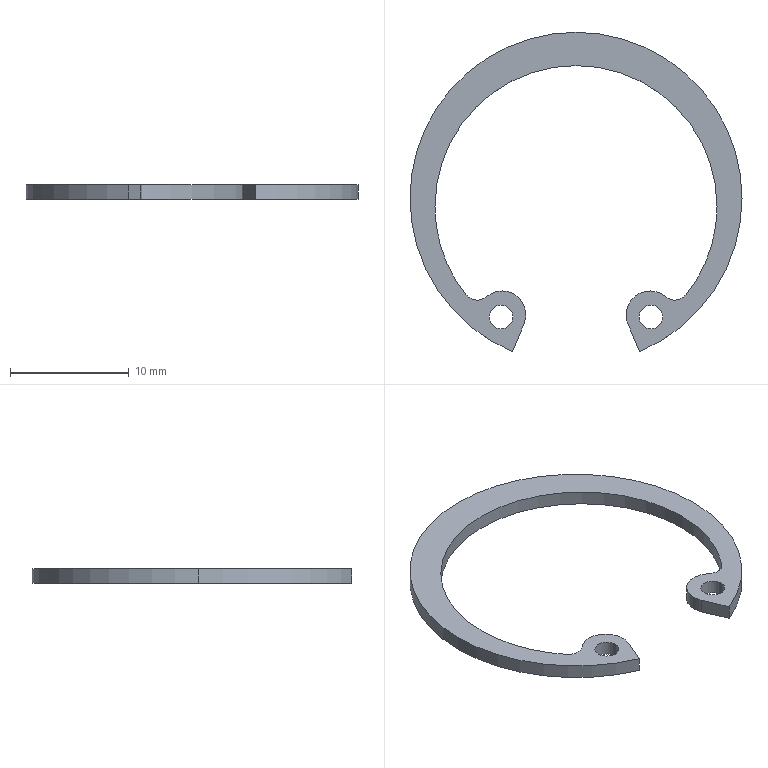Part | NX | features BREP 1 | 1 solid | 19 faces | box 27.9 x 26.838 x 1.2 mm | volume 202.858 mm3 | cylinder 15 | plane 4 | commonest cylinder face diameters 2 x4 4 x3 23.7 x3 27.9 x3 2.4 x2
STEP:
#1=CARTESIAN_POINT('',(-4.369,-10.547,-0.6));
#2=VERTEX_POINT('',#1);
#3=CARTESIAN_POINT('',(-7.525,-8.269,-0.6));
#4=VERTEX_POINT('',#3);
#5=CARTESIAN_POINT('',(-6.217,-9.782,-0.6));
#6=DIRECTION('',(0.,0.,1.));
#7=DIRECTION('',(1.,0.,0.));
#8=AXIS2_PLACEMENT_3D('',#5,#6,#7);
#9=CIRCLE('',#8,2.);
#10=EDGE_CURVE('',#2,#4,#9,.T.);
#11=ORIENTED_EDGE('',*,*,#10,.F.);
#12=CARTESIAN_POINT('',(-5.338,-12.888,-0.6));
#13=VERTEX_POINT('',#12);
#14=CARTESIAN_POINT('',(-4.369,-10.547,-0.6));
#15=DIRECTION('',(0.3827,0.9239,0.));
#16=VECTOR('',#15,1000.);
#17=LINE('',#14,#16);
#18=EDGE_CURVE('',#13,#2,#17,.T.);
#19=ORIENTED_EDGE('',*,*,#18,.F.);
#20=CARTESIAN_POINT('',(-13.95,0.,-0.6));
#21=VERTEX_POINT('',#20);
#22=CARTESIAN_POINT('',(0.,0.,-0.6));
#23=DIRECTION('',(0.,0.,1.));
#24=DIRECTION('',(1.,0.,0.));
#25=AXIS2_PLACEMENT_3D('',#22,#23,#24);
#26=CIRCLE('',#25,13.95);
#27=EDGE_CURVE('',#21,#13,#26,.T.);
#28=ORIENTED_EDGE('',*,*,#27,.F.);
#29=CARTESIAN_POINT('',(13.95,0.,-0.6));
#30=VERTEX_POINT('',#29);
#31=CARTESIAN_POINT('',(0.,0.,-0.6));
#32=DIRECTION('',(0.,0.,1.));
#33=DIRECTION('',(1.,0.,0.));
#34=AXIS2_PLACEMENT_3D('',#31,#32,#33);
#35=CIRCLE('',#34,13.95);
#36=EDGE_CURVE('',#30,#21,#35,.T.);
#37=ORIENTED_EDGE('',*,*,#36,.F.);
#38=CARTESIAN_POINT('',(5.338,-12.888,-0.6));
#39=VERTEX_POINT('',#38);
#40=CARTESIAN_POINT('',(0.,0.,-0.6));
#41=DIRECTION('',(0.,0.,1.));
#42=DIRECTION('',(1.,0.,0.));
#43=AXIS2_PLACEMENT_3D('',#40,#41,#42);
#44=CIRCLE('',#43,13.95);
#45=EDGE_CURVE('',#39,#30,#44,.T.);
#46=ORIENTED_EDGE('',*,*,#45,.F.);
#47=CARTESIAN_POINT('',(4.369,-10.547,-0.6));
#48=VERTEX_POINT('',#47);
#49=CARTESIAN_POINT('',(4.369,-10.547,-0.6));
#50=DIRECTION('',(0.3827,-0.9239,0.));
#51=VECTOR('',#50,1000.);
#52=LINE('',#49,#51);
#53=EDGE_CURVE('',#48,#39,#52,.T.);
#54=ORIENTED_EDGE('',*,*,#53,.F.);
#55=CARTESIAN_POINT('',(4.217,-9.782,-0.6));
#56=VERTEX_POINT('',#55);
#57=CARTESIAN_POINT('',(6.217,-9.782,-0.6));
#58=DIRECTION('',(0.,0.,1.));
#59=DIRECTION('',(-1.,0.,0.));
#60=AXIS2_PLACEMENT_3D('',#57,#58,#59);
#61=CIRCLE('',#60,2.);
#62=EDGE_CURVE('',#56,#48,#61,.T.);
#63=ORIENTED_EDGE('',*,*,#62,.F.);
#64=CARTESIAN_POINT('',(7.525,-8.269,-0.6));
#65=VERTEX_POINT('',#64);
#66=CARTESIAN_POINT('',(6.217,-9.782,-0.6));
#67=DIRECTION('',(0.,0.,1.));
#68=DIRECTION('',(-1.,0.,0.));
#69=AXIS2_PLACEMENT_3D('',#66,#67,#68);
#70=CIRCLE('',#69,2.);
#71=EDGE_CURVE('',#65,#56,#70,.T.);
#72=ORIENTED_EDGE('',*,*,#71,.F.);
#73=CARTESIAN_POINT('',(9.246,-8.112,-0.6));
#74=VERTEX_POINT('',#73);
#75=CARTESIAN_POINT('',(8.31,-7.361,-0.6));
#76=DIRECTION('',(0.,0.,-1.));
#77=DIRECTION('',(1.,0.,0.));
#78=AXIS2_PLACEMENT_3D('',#75,#76,#77);
#79=CIRCLE('',#78,1.2);
#80=EDGE_CURVE('',#74,#65,#79,.T.);
#81=ORIENTED_EDGE('',*,*,#80,.F.);
#82=CARTESIAN_POINT('',(11.85,-0.7,-0.6));
#83=VERTEX_POINT('',#82);
#84=CARTESIAN_POINT('',(0.,-0.7,-0.6));
#85=DIRECTION('',(0.,0.,-1.));
#86=DIRECTION('',(1.,0.,0.));
#87=AXIS2_PLACEMENT_3D('',#84,#85,#86);
#88=CIRCLE('',#87,11.85);
#89=EDGE_CURVE('',#83,#74,#88,.T.);
#90=ORIENTED_EDGE('',*,*,#89,.F.);
#91=CARTESIAN_POINT('',(-11.85,-0.7,-0.6));
#92=VERTEX_POINT('',#91);
#93=CARTESIAN_POINT('',(0.,-0.7,-0.6));
#94=DIRECTION('',(0.,0.,-1.));
#95=DIRECTION('',(1.,0.,0.));
#96=AXIS2_PLACEMENT_3D('',#93,#94,#95);
#97=CIRCLE('',#96,11.85);
#98=EDGE_CURVE('',#92,#83,#97,.T.);
#99=ORIENTED_EDGE('',*,*,#98,.F.);
#100=CARTESIAN_POINT('',(-9.246,-8.112,-0.6));
#101=VERTEX_POINT('',#100);
#102=CARTESIAN_POINT('',(0.,-0.7,-0.6));
#103=DIRECTION('',(0.,0.,-1.));
#104=DIRECTION('',(1.,0.,0.));
#105=AXIS2_PLACEMENT_3D('',#102,#103,#104);
#106=CIRCLE('',#105,11.85);
#107=EDGE_CURVE('',#101,#92,#106,.T.);
#108=ORIENTED_EDGE('',*,*,#107,.F.);
#109=CARTESIAN_POINT('',(-8.31,-7.361,-0.6));
#110=DIRECTION('',(0.,0.,-1.));
#111=DIRECTION('',(-1.,0.,0.));
#112=AXIS2_PLACEMENT_3D('',#109,#110,#111);
#113=CIRCLE('',#112,1.2);
#114=EDGE_CURVE('',#4,#101,#113,.T.);
#115=ORIENTED_EDGE('',*,*,#114,.F.);
#116=EDGE_LOOP('',(#11,#19,#28,#37,#46,#54,#63,#72,#81,#90,#99,#108,#115));
#117=FACE_BOUND('',#116,.T.);
#118=CARTESIAN_POINT('',(-7.298,-9.979,-0.6));
#119=VERTEX_POINT('',#118);
#120=CARTESIAN_POINT('',(-5.298,-9.979,-0.6));
#121=VERTEX_POINT('',#120);
#122=CARTESIAN_POINT('',(-6.298,-9.979,-0.6));
#123=DIRECTION('',(0.,0.,1.));
#124=DIRECTION('',(1.,0.,0.));
#125=AXIS2_PLACEMENT_3D('',#122,#123,#124);
#126=CIRCLE('',#125,1.);
#127=EDGE_CURVE('',#119,#121,#126,.T.);
#128=ORIENTED_EDGE('',*,*,#127,.T.);
#129=CARTESIAN_POINT('',(-6.298,-9.979,-0.6));
#130=DIRECTION('',(0.,0.,1.));
#131=DIRECTION('',(1.,0.,0.));
#132=AXIS2_PLACEMENT_3D('',#129,#130,#131);
#133=CIRCLE('',#132,1.);
#134=EDGE_CURVE('',#121,#119,#133,.T.);
#135=ORIENTED_EDGE('',*,*,#134,.T.);
#136=EDGE_LOOP('',(#128,#135));
#137=FACE_BOUND('',#136,.T.);
#138=CARTESIAN_POINT('',(5.298,-9.979,-0.6));
#139=VERTEX_POINT('',#138);
#140=CARTESIAN_POINT('',(7.298,-9.979,-0.6));
#141=VERTEX_POINT('',#140);
#142=CARTESIAN_POINT('',(6.298,-9.979,-0.6));
#143=DIRECTION('',(0.,0.,1.));
#144=DIRECTION('',(-1.,0.,0.));
#145=AXIS2_PLACEMENT_3D('',#142,#143,#144);
#146=CIRCLE('',#145,1.);
#147=EDGE_CURVE('',#139,#141,#146,.T.);
#148=ORIENTED_EDGE('',*,*,#147,.T.);
#149=CARTESIAN_POINT('',(6.298,-9.979,-0.6));
#150=DIRECTION('',(0.,0.,1.));
#151=DIRECTION('',(-1.,0.,0.));
#152=AXIS2_PLACEMENT_3D('',#149,#150,#151);
#153=CIRCLE('',#152,1.);
#154=EDGE_CURVE('',#141,#139,#153,.T.);
#155=ORIENTED_EDGE('',*,*,#154,.T.);
#156=EDGE_LOOP('',(#148,#155));
#157=FACE_BOUND('',#156,.T.);
#158=CARTESIAN_POINT('',(-6.217,-9.782,-0.6));
#159=DIRECTION('',(0.,0.,1.));
#160=DIRECTION('',(1.,0.,0.));
#161=AXIS2_PLACEMENT_3D('',#158,#159,#160);
#162=PLANE('',#161);
#163=ADVANCED_FACE('',(#117,#137,#157),#162,.F.);
#164=CARTESIAN_POINT('',(7.298,-9.979,0.6));
#165=VERTEX_POINT('',#164);
#166=CARTESIAN_POINT('',(7.298,-9.979,0.6));
#167=DIRECTION('',(0.,0.,-1.));
#168=VECTOR('',#167,1000.);
#169=LINE('',#166,#168);
#170=EDGE_CURVE('',#165,#141,#169,.T.);
#171=ORIENTED_EDGE('',*,*,#170,.F.);
#172=CARTESIAN_POINT('',(5.298,-9.979,0.6));
#173=VERTEX_POINT('',#172);
#174=CARTESIAN_POINT('',(6.298,-9.979,0.6));
#175=DIRECTION('',(0.,0.,1.));
#176=DIRECTION('',(-1.,0.,0.));
#177=AXIS2_PLACEMENT_3D('',#174,#175,#176);
#178=CIRCLE('',#177,1.);
#179=EDGE_CURVE('',#165,#173,#178,.T.);
#180=ORIENTED_EDGE('',*,*,#179,.T.);
#181=CARTESIAN_POINT('',(5.298,-9.979,0.6));
#182=DIRECTION('',(0.,0.,-1.));
#183=VECTOR('',#182,1000.);
#184=LINE('',#181,#183);
#185=EDGE_CURVE('',#173,#139,#184,.T.);
#186=ORIENTED_EDGE('',*,*,#185,.T.);
#187=ORIENTED_EDGE('',*,*,#154,.F.);
#188=EDGE_LOOP('',(#171,#180,#186,#187));
#189=FACE_BOUND('',#188,.T.);
#190=CARTESIAN_POINT('',(6.298,-9.979,0.6));
#191=DIRECTION('',(0.,0.,-1.));
#192=DIRECTION('',(-1.,0.,0.));
#193=AXIS2_PLACEMENT_3D('',#190,#191,#192);
#194=CYLINDRICAL_SURFACE('',#193,1.);
#195=ADVANCED_FACE('',(#189),#194,.F.);
#196=CARTESIAN_POINT('',(-5.298,-9.979,0.6));
#197=VERTEX_POINT('',#196);
#198=CARTESIAN_POINT('',(-5.298,-9.979,0.6));
#199=DIRECTION('',(0.,0.,-1.));
#200=VECTOR('',#199,1000.);
#201=LINE('',#198,#200);
#202=EDGE_CURVE('',#197,#121,#201,.T.);
#203=ORIENTED_EDGE('',*,*,#202,.F.);
#204=CARTESIAN_POINT('',(-7.298,-9.979,0.6));
#205=VERTEX_POINT('',#204);
#206=CARTESIAN_POINT('',(-6.298,-9.979,0.6));
#207=DIRECTION('',(0.,0.,1.));
#208=DIRECTION('',(1.,0.,0.));
#209=AXIS2_PLACEMENT_3D('',#206,#207,#208);
#210=CIRCLE('',#209,1.);
#211=EDGE_CURVE('',#197,#205,#210,.T.);
#212=ORIENTED_EDGE('',*,*,#211,.T.);
#213=CARTESIAN_POINT('',(-7.298,-9.979,0.6));
#214=DIRECTION('',(0.,0.,-1.));
#215=VECTOR('',#214,1000.);
#216=LINE('',#213,#215);
#217=EDGE_CURVE('',#205,#119,#216,.T.);
#218=ORIENTED_EDGE('',*,*,#217,.T.);
#219=ORIENTED_EDGE('',*,*,#134,.F.);
#220=EDGE_LOOP('',(#203,#212,#218,#219));
#221=FACE_BOUND('',#220,.T.);
#222=CARTESIAN_POINT('',(-6.298,-9.979,0.6));
#223=DIRECTION('',(0.,0.,-1.));
#224=DIRECTION('',(-1.,0.,0.));
#225=AXIS2_PLACEMENT_3D('',#222,#223,#224);
#226=CYLINDRICAL_SURFACE('',#225,1.);
#227=ADVANCED_FACE('',(#221),#226,.F.);
#228=CARTESIAN_POINT('',(-5.338,-12.888,0.6));
#229=VERTEX_POINT('',#228);
#230=CARTESIAN_POINT('',(-5.338,-12.888,0.6));
#231=DIRECTION('',(0.,0.,-1.));
#232=VECTOR('',#231,1000.);
#233=LINE('',#230,#232);
#234=EDGE_CURVE('',#229,#13,#233,.T.);
#235=ORIENTED_EDGE('',*,*,#234,.T.);
#236=ORIENTED_EDGE('',*,*,#18,.T.);
#237=CARTESIAN_POINT('',(-4.369,-10.547,0.6));
#238=VERTEX_POINT('',#237);
#239=CARTESIAN_POINT('',(-4.369,-10.547,0.6));
#240=DIRECTION('',(0.,0.,-1.));
#241=VECTOR('',#240,1000.);
#242=LINE('',#239,#241);
#243=EDGE_CURVE('',#238,#2,#242,.T.);
#244=ORIENTED_EDGE('',*,*,#243,.F.);
#245=CARTESIAN_POINT('',(-4.369,-10.547,0.6));
#246=DIRECTION('',(0.3827,0.9239,0.));
#247=VECTOR('',#246,1000.);
#248=LINE('',#245,#247);
#249=EDGE_CURVE('',#229,#238,#248,.T.);
#250=ORIENTED_EDGE('',*,*,#249,.F.);
#251=EDGE_LOOP('',(#235,#236,#244,#250));
#252=FACE_BOUND('',#251,.T.);
#253=CARTESIAN_POINT('',(-4.369,-10.547,0.6));
#254=DIRECTION('',(-0.9239,0.3827,0.));
#255=DIRECTION('',(-0.3827,-0.9239,0.));
#256=AXIS2_PLACEMENT_3D('',#253,#254,#255);
#257=PLANE('',#256);
#258=ADVANCED_FACE('',(#252),#257,.F.);
#259=CARTESIAN_POINT('',(13.95,0.,0.6));
#260=VERTEX_POINT('',#259);
#261=CARTESIAN_POINT('',(13.95,0.,0.6));
#262=DIRECTION('',(0.,0.,-1.));
#263=VECTOR('',#262,1000.);
#264=LINE('',#261,#263);
#265=EDGE_CURVE('',#260,#30,#264,.T.);
#266=ORIENTED_EDGE('',*,*,#265,.F.);
#267=CARTESIAN_POINT('',(5.338,-12.888,0.6));
#268=VERTEX_POINT('',#267);
#269=CARTESIAN_POINT('',(0.,0.,0.6));
#270=DIRECTION('',(0.,0.,1.));
#271=DIRECTION('',(1.,0.,0.));
#272=AXIS2_PLACEMENT_3D('',#269,#270,#271);
#273=CIRCLE('',#272,13.95);
#274=EDGE_CURVE('',#268,#260,#273,.T.);
#275=ORIENTED_EDGE('',*,*,#274,.F.);
#276=CARTESIAN_POINT('',(5.338,-12.888,0.6));
#277=DIRECTION('',(0.,0.,-1.));
#278=VECTOR('',#277,1000.);
#279=LINE('',#276,#278);
#280=EDGE_CURVE('',#268,#39,#279,.T.);
#281=ORIENTED_EDGE('',*,*,#280,.T.);
#282=ORIENTED_EDGE('',*,*,#45,.T.);
#283=EDGE_LOOP('',(#266,#275,#281,#282));
#284=FACE_BOUND('',#283,.T.);
#285=CARTESIAN_POINT('',(0.,0.,0.6));
#286=DIRECTION('',(0.,0.,-1.));
#287=DIRECTION('',(-1.,0.,0.));
#288=AXIS2_PLACEMENT_3D('',#285,#286,#287);
#289=CYLINDRICAL_SURFACE('',#288,13.95);
#290=ADVANCED_FACE('',(#284),#289,.T.);
#291=CARTESIAN_POINT('',(4.369,-10.547,0.6));
#292=VERTEX_POINT('',#291);
#293=CARTESIAN_POINT('',(4.369,-10.547,0.6));
#294=DIRECTION('',(0.,0.,-1.));
#295=VECTOR('',#294,1000.);
#296=LINE('',#293,#295);
#297=EDGE_CURVE('',#292,#48,#296,.T.);
#298=ORIENTED_EDGE('',*,*,#297,.T.);
#299=ORIENTED_EDGE('',*,*,#53,.T.);
#300=ORIENTED_EDGE('',*,*,#280,.F.);
#301=CARTESIAN_POINT('',(4.369,-10.547,0.6));
#302=DIRECTION('',(0.3827,-0.9239,0.));
#303=VECTOR('',#302,1000.);
#304=LINE('',#301,#303);
#305=EDGE_CURVE('',#292,#268,#304,.T.);
#306=ORIENTED_EDGE('',*,*,#305,.F.);
#307=EDGE_LOOP('',(#298,#299,#300,#306));
#308=FACE_BOUND('',#307,.T.);
#309=CARTESIAN_POINT('',(4.369,-10.547,0.6));
#310=DIRECTION('',(0.9239,0.3827,0.));
#311=DIRECTION('',(-0.3827,0.9239,0.));
#312=AXIS2_PLACEMENT_3D('',#309,#310,#311);
#313=PLANE('',#312);
#314=ADVANCED_FACE('',(#308),#313,.F.);
#315=CARTESIAN_POINT('',(4.217,-9.782,0.6));
#316=VERTEX_POINT('',#315);
#317=CARTESIAN_POINT('',(4.217,-9.782,0.6));
#318=DIRECTION('',(0.,0.,-1.));
#319=VECTOR('',#318,1000.);
#320=LINE('',#317,#319);
#321=EDGE_CURVE('',#316,#56,#320,.T.);
#322=ORIENTED_EDGE('',*,*,#321,.F.);
#323=CARTESIAN_POINT('',(7.525,-8.269,0.6));
#324=VERTEX_POINT('',#323);
#325=CARTESIAN_POINT('',(6.217,-9.782,0.6));
#326=DIRECTION('',(0.,0.,1.));
#327=DIRECTION('',(-1.,0.,0.));
#328=AXIS2_PLACEMENT_3D('',#325,#326,#327);
#329=CIRCLE('',#328,2.);
#330=EDGE_CURVE('',#324,#316,#329,.T.);
#331=ORIENTED_EDGE('',*,*,#330,.F.);
#332=CARTESIAN_POINT('',(7.525,-8.269,0.6));
#333=DIRECTION('',(0.,0.,-1.));
#334=VECTOR('',#333,1000.);
#335=LINE('',#332,#334);
#336=EDGE_CURVE('',#324,#65,#335,.T.);
#337=ORIENTED_EDGE('',*,*,#336,.T.);
#338=ORIENTED_EDGE('',*,*,#71,.T.);
#339=EDGE_LOOP('',(#322,#331,#337,#338));
#340=FACE_BOUND('',#339,.T.);
#341=CARTESIAN_POINT('',(6.217,-9.782,0.6));
#342=DIRECTION('',(0.,0.,-1.));
#343=DIRECTION('',(-1.,0.,0.));
#344=AXIS2_PLACEMENT_3D('',#341,#342,#343);
#345=CYLINDRICAL_SURFACE('',#344,2.);
#346=ADVANCED_FACE('',(#340),#345,.T.);
#347=CARTESIAN_POINT('',(9.246,-8.112,0.6));
#348=VERTEX_POINT('',#347);
#349=CARTESIAN_POINT('',(9.246,-8.112,0.6));
#350=DIRECTION('',(0.,0.,-1.));
#351=VECTOR('',#350,1000.);
#352=LINE('',#349,#351);
#353=EDGE_CURVE('',#348,#74,#352,.T.);
#354=ORIENTED_EDGE('',*,*,#353,.T.);
#355=ORIENTED_EDGE('',*,*,#80,.T.);
#356=ORIENTED_EDGE('',*,*,#336,.F.);
#357=CARTESIAN_POINT('',(8.31,-7.361,0.6));
#358=DIRECTION('',(0.,0.,-1.));
#359=DIRECTION('',(1.,0.,0.));
#360=AXIS2_PLACEMENT_3D('',#357,#358,#359);
#361=CIRCLE('',#360,1.2);
#362=EDGE_CURVE('',#348,#324,#361,.T.);
#363=ORIENTED_EDGE('',*,*,#362,.F.);
#364=EDGE_LOOP('',(#354,#355,#356,#363));
#365=FACE_BOUND('',#364,.T.);
#366=CARTESIAN_POINT('',(8.31,-7.361,0.6));
#367=DIRECTION('',(0.,0.,-1.));
#368=DIRECTION('',(-1.,0.,0.));
#369=AXIS2_PLACEMENT_3D('',#366,#367,#368);
#370=CYLINDRICAL_SURFACE('',#369,1.2);
#371=ADVANCED_FACE('',(#365),#370,.F.);
#372=CARTESIAN_POINT('',(-11.85,-0.7,0.6));
#373=VERTEX_POINT('',#372);
#374=CARTESIAN_POINT('',(-11.85,-0.7,0.6));
#375=DIRECTION('',(0.,0.,-1.));
#376=VECTOR('',#375,1000.);
#377=LINE('',#374,#376);
#378=EDGE_CURVE('',#373,#92,#377,.T.);
#379=ORIENTED_EDGE('',*,*,#378,.F.);
#380=CARTESIAN_POINT('',(-9.246,-8.112,0.6));
#381=VERTEX_POINT('',#380);
#382=CARTESIAN_POINT('',(0.,-0.7,0.6));
#383=DIRECTION('',(0.,0.,-1.));
#384=DIRECTION('',(1.,0.,0.));
#385=AXIS2_PLACEMENT_3D('',#382,#383,#384);
#386=CIRCLE('',#385,11.85);
#387=EDGE_CURVE('',#381,#373,#386,.T.);
#388=ORIENTED_EDGE('',*,*,#387,.F.);
#389=CARTESIAN_POINT('',(-9.246,-8.112,0.6));
#390=DIRECTION('',(0.,0.,-1.));
#391=VECTOR('',#390,1000.);
#392=LINE('',#389,#391);
#393=EDGE_CURVE('',#381,#101,#392,.T.);
#394=ORIENTED_EDGE('',*,*,#393,.T.);
#395=ORIENTED_EDGE('',*,*,#107,.T.);
#396=EDGE_LOOP('',(#379,#388,#394,#395));
#397=FACE_BOUND('',#396,.T.);
#398=CARTESIAN_POINT('',(0.,-0.7,0.6));
#399=DIRECTION('',(0.,0.,-1.));
#400=DIRECTION('',(-1.,0.,0.));
#401=AXIS2_PLACEMENT_3D('',#398,#399,#400);
#402=CYLINDRICAL_SURFACE('',#401,11.85);
#403=ADVANCED_FACE('',(#397),#402,.F.);
#404=CARTESIAN_POINT('',(-7.525,-8.269,0.6));
#405=VERTEX_POINT('',#404);
#406=CARTESIAN_POINT('',(-7.525,-8.269,0.6));
#407=DIRECTION('',(0.,0.,-1.));
#408=VECTOR('',#407,1000.);
#409=LINE('',#406,#408);
#410=EDGE_CURVE('',#405,#4,#409,.T.);
#411=ORIENTED_EDGE('',*,*,#410,.T.);
#412=ORIENTED_EDGE('',*,*,#114,.T.);
#413=ORIENTED_EDGE('',*,*,#393,.F.);
#414=CARTESIAN_POINT('',(-8.31,-7.361,0.6));
#415=DIRECTION('',(0.,0.,-1.));
#416=DIRECTION('',(-1.,0.,0.));
#417=AXIS2_PLACEMENT_3D('',#414,#415,#416);
#418=CIRCLE('',#417,1.2);
#419=EDGE_CURVE('',#405,#381,#418,.T.);
#420=ORIENTED_EDGE('',*,*,#419,.F.);
#421=EDGE_LOOP('',(#411,#412,#413,#420));
#422=FACE_BOUND('',#421,.T.);
#423=CARTESIAN_POINT('',(-8.31,-7.361,0.6));
#424=DIRECTION('',(0.,0.,-1.));
#425=DIRECTION('',(-1.,0.,0.));
#426=AXIS2_PLACEMENT_3D('',#423,#424,#425);
#427=CYLINDRICAL_SURFACE('',#426,1.2);
#428=ADVANCED_FACE('',(#422),#427,.F.);
#429=ORIENTED_EDGE('',*,*,#243,.T.);
#430=ORIENTED_EDGE('',*,*,#10,.T.);
#431=ORIENTED_EDGE('',*,*,#410,.F.);
#432=CARTESIAN_POINT('',(-6.217,-9.782,0.6));
#433=DIRECTION('',(0.,0.,1.));
#434=DIRECTION('',(1.,0.,0.));
#435=AXIS2_PLACEMENT_3D('',#432,#433,#434);
#436=CIRCLE('',#435,2.);
#437=EDGE_CURVE('',#238,#405,#436,.T.);
#438=ORIENTED_EDGE('',*,*,#437,.F.);
#439=EDGE_LOOP('',(#429,#430,#431,#438));
#440=FACE_BOUND('',#439,.T.);
#441=CARTESIAN_POINT('',(-6.217,-9.782,0.6));
#442=DIRECTION('',(0.,0.,-1.));
#443=DIRECTION('',(-1.,0.,0.));
#444=AXIS2_PLACEMENT_3D('',#441,#442,#443);
#445=CYLINDRICAL_SURFACE('',#444,2.);
#446=ADVANCED_FACE('',(#440),#445,.T.);
#447=CARTESIAN_POINT('',(6.298,-9.979,0.6));
#448=DIRECTION('',(0.,0.,1.));
#449=DIRECTION('',(-1.,0.,0.));
#450=AXIS2_PLACEMENT_3D('',#447,#448,#449);
#451=CIRCLE('',#450,1.);
#452=EDGE_CURVE('',#173,#165,#451,.T.);
#453=ORIENTED_EDGE('',*,*,#452,.F.);
#454=ORIENTED_EDGE('',*,*,#179,.F.);
#455=EDGE_LOOP('',(#453,#454));
#456=FACE_BOUND('',#455,.T.);
#457=ORIENTED_EDGE('',*,*,#437,.T.);
#458=ORIENTED_EDGE('',*,*,#419,.T.);
#459=ORIENTED_EDGE('',*,*,#387,.T.);
#460=CARTESIAN_POINT('',(11.85,-0.7,0.6));
#461=VERTEX_POINT('',#460);
#462=CARTESIAN_POINT('',(0.,-0.7,0.6));
#463=DIRECTION('',(0.,0.,-1.));
#464=DIRECTION('',(1.,0.,0.));
#465=AXIS2_PLACEMENT_3D('',#462,#463,#464);
#466=CIRCLE('',#465,11.85);
#467=EDGE_CURVE('',#373,#461,#466,.T.);
#468=ORIENTED_EDGE('',*,*,#467,.T.);
#469=CARTESIAN_POINT('',(0.,-0.7,0.6));
#470=DIRECTION('',(0.,0.,-1.));
#471=DIRECTION('',(1.,0.,0.));
#472=AXIS2_PLACEMENT_3D('',#469,#470,#471);
#473=CIRCLE('',#472,11.85);
#474=EDGE_CURVE('',#461,#348,#473,.T.);
#475=ORIENTED_EDGE('',*,*,#474,.T.);
#476=ORIENTED_EDGE('',*,*,#362,.T.);
#477=ORIENTED_EDGE('',*,*,#330,.T.);
#478=CARTESIAN_POINT('',(6.217,-9.782,0.6));
#479=DIRECTION('',(0.,0.,1.));
#480=DIRECTION('',(-1.,0.,0.));
#481=AXIS2_PLACEMENT_3D('',#478,#479,#480);
#482=CIRCLE('',#481,2.);
#483=EDGE_CURVE('',#316,#292,#482,.T.);
#484=ORIENTED_EDGE('',*,*,#483,.T.);
#485=ORIENTED_EDGE('',*,*,#305,.T.);
#486=ORIENTED_EDGE('',*,*,#274,.T.);
#487=CARTESIAN_POINT('',(-13.95,0.,0.6));
#488=VERTEX_POINT('',#487);
#489=CARTESIAN_POINT('',(0.,0.,0.6));
#490=DIRECTION('',(0.,0.,1.));
#491=DIRECTION('',(1.,0.,0.));
#492=AXIS2_PLACEMENT_3D('',#489,#490,#491);
#493=CIRCLE('',#492,13.95);
#494=EDGE_CURVE('',#260,#488,#493,.T.);
#495=ORIENTED_EDGE('',*,*,#494,.T.);
#496=CARTESIAN_POINT('',(0.,0.,0.6));
#497=DIRECTION('',(0.,0.,1.));
#498=DIRECTION('',(1.,0.,0.));
#499=AXIS2_PLACEMENT_3D('',#496,#497,#498);
#500=CIRCLE('',#499,13.95);
#501=EDGE_CURVE('',#488,#229,#500,.T.);
#502=ORIENTED_EDGE('',*,*,#501,.T.);
#503=ORIENTED_EDGE('',*,*,#249,.T.);
#504=EDGE_LOOP('',(#457,#458,#459,#468,#475,#476,#477,#484,#485,#486,#495,#502,#503));
#505=FACE_BOUND('',#504,.T.);
#506=CARTESIAN_POINT('',(-6.298,-9.979,0.6));
#507=DIRECTION('',(0.,0.,1.));
#508=DIRECTION('',(1.,0.,0.));
#509=AXIS2_PLACEMENT_3D('',#506,#507,#508);
#510=CIRCLE('',#509,1.);
#511=EDGE_CURVE('',#205,#197,#510,.T.);
#512=ORIENTED_EDGE('',*,*,#511,.F.);
#513=ORIENTED_EDGE('',*,*,#211,.F.);
#514=EDGE_LOOP('',(#512,#513));
#515=FACE_BOUND('',#514,.T.);
#516=CARTESIAN_POINT('',(-6.217,-9.782,0.6));
#517=DIRECTION('',(0.,0.,1.));
#518=DIRECTION('',(1.,0.,0.));
#519=AXIS2_PLACEMENT_3D('',#516,#517,#518);
#520=PLANE('',#519);
#521=ADVANCED_FACE('',(#456,#505,#515),#520,.T.);
#522=CARTESIAN_POINT('',(11.85,-0.7,0.6));
#523=DIRECTION('',(0.,0.,-1.));
#524=VECTOR('',#523,1000.);
#525=LINE('',#522,#524);
#526=EDGE_CURVE('',#461,#83,#525,.T.);
#527=ORIENTED_EDGE('',*,*,#526,.F.);
#528=ORIENTED_EDGE('',*,*,#467,.F.);
#529=ORIENTED_EDGE('',*,*,#378,.T.);
#530=ORIENTED_EDGE('',*,*,#98,.T.);
#531=EDGE_LOOP('',(#527,#528,#529,#530));
#532=FACE_BOUND('',#531,.T.);
#533=CARTESIAN_POINT('',(0.,-0.7,0.6));
#534=DIRECTION('',(0.,0.,-1.));
#535=DIRECTION('',(-1.,0.,0.));
#536=AXIS2_PLACEMENT_3D('',#533,#534,#535);
#537=CYLINDRICAL_SURFACE('',#536,11.85);
#538=ADVANCED_FACE('',(#532),#537,.F.);
#539=ORIENTED_EDGE('',*,*,#474,.F.);
#540=ORIENTED_EDGE('',*,*,#526,.T.);
#541=ORIENTED_EDGE('',*,*,#89,.T.);
#542=ORIENTED_EDGE('',*,*,#353,.F.);
#543=EDGE_LOOP('',(#539,#540,#541,#542));
#544=FACE_BOUND('',#543,.T.);
#545=CARTESIAN_POINT('',(0.,-0.7,0.6));
#546=DIRECTION('',(0.,0.,-1.));
#547=DIRECTION('',(-1.,0.,0.));
#548=AXIS2_PLACEMENT_3D('',#545,#546,#547);
#549=CYLINDRICAL_SURFACE('',#548,11.85);
#550=ADVANCED_FACE('',(#544),#549,.F.);
#551=ORIENTED_EDGE('',*,*,#483,.F.);
#552=ORIENTED_EDGE('',*,*,#321,.T.);
#553=ORIENTED_EDGE('',*,*,#62,.T.);
#554=ORIENTED_EDGE('',*,*,#297,.F.);
#555=EDGE_LOOP('',(#551,#552,#553,#554));
#556=FACE_BOUND('',#555,.T.);
#557=CARTESIAN_POINT('',(6.217,-9.782,0.6));
#558=DIRECTION('',(0.,0.,-1.));
#559=DIRECTION('',(-1.,0.,0.));
#560=AXIS2_PLACEMENT_3D('',#557,#558,#559);
#561=CYLINDRICAL_SURFACE('',#560,2.);
#562=ADVANCED_FACE('',(#556),#561,.T.);
#563=ORIENTED_EDGE('',*,*,#501,.F.);
#564=CARTESIAN_POINT('',(-13.95,0.,0.6));
#565=DIRECTION('',(0.,0.,-1.));
#566=VECTOR('',#565,1000.);
#567=LINE('',#564,#566);
#568=EDGE_CURVE('',#488,#21,#567,.T.);
#569=ORIENTED_EDGE('',*,*,#568,.T.);
#570=ORIENTED_EDGE('',*,*,#27,.T.);
#571=ORIENTED_EDGE('',*,*,#234,.F.);
#572=EDGE_LOOP('',(#563,#569,#570,#571));
#573=FACE_BOUND('',#572,.T.);
#574=CARTESIAN_POINT('',(0.,0.,0.6));
#575=DIRECTION('',(0.,0.,-1.));
#576=DIRECTION('',(-1.,0.,0.));
#577=AXIS2_PLACEMENT_3D('',#574,#575,#576);
#578=CYLINDRICAL_SURFACE('',#577,13.95);
#579=ADVANCED_FACE('',(#573),#578,.T.);
#580=ORIENTED_EDGE('',*,*,#494,.F.);
#581=ORIENTED_EDGE('',*,*,#265,.T.);
#582=ORIENTED_EDGE('',*,*,#36,.T.);
#583=ORIENTED_EDGE('',*,*,#568,.F.);
#584=EDGE_LOOP('',(#580,#581,#582,#583));
#585=FACE_BOUND('',#584,.T.);
#586=CARTESIAN_POINT('',(0.,0.,0.6));
#587=DIRECTION('',(0.,0.,-1.));
#588=DIRECTION('',(-1.,0.,0.));
#589=AXIS2_PLACEMENT_3D('',#586,#587,#588);
#590=CYLINDRICAL_SURFACE('',#589,13.95);
#591=ADVANCED_FACE('',(#585),#590,.T.);
#592=ORIENTED_EDGE('',*,*,#511,.T.);
#593=ORIENTED_EDGE('',*,*,#202,.T.);
#594=ORIENTED_EDGE('',*,*,#127,.F.);
#595=ORIENTED_EDGE('',*,*,#217,.F.);
#596=EDGE_LOOP('',(#592,#593,#594,#595));
#597=FACE_BOUND('',#596,.T.);
#598=CARTESIAN_POINT('',(-6.298,-9.979,0.6));
#599=DIRECTION('',(0.,0.,-1.));
#600=DIRECTION('',(-1.,0.,0.));
#601=AXIS2_PLACEMENT_3D('',#598,#599,#600);
#602=CYLINDRICAL_SURFACE('',#601,1.);
#603=ADVANCED_FACE('',(#597),#602,.F.);
#604=ORIENTED_EDGE('',*,*,#452,.T.);
#605=ORIENTED_EDGE('',*,*,#170,.T.);
#606=ORIENTED_EDGE('',*,*,#147,.F.);
#607=ORIENTED_EDGE('',*,*,#185,.F.);
#608=EDGE_LOOP('',(#604,#605,#606,#607));
#609=FACE_BOUND('',#608,.T.);
#610=CARTESIAN_POINT('',(6.298,-9.979,0.6));
#611=DIRECTION('',(0.,0.,-1.));
#612=DIRECTION('',(-1.,0.,0.));
#613=AXIS2_PLACEMENT_3D('',#610,#611,#612);
#614=CYLINDRICAL_SURFACE('',#613,1.);
#615=ADVANCED_FACE('',(#609),#614,.F.);
#616=CLOSED_SHELL('',(#163,#195,#227,#258,#290,#314,#346,#371,#403,#428,#446,#521,#538,#550,#562,#579,#591,#603,#615));
#617=MANIFOLD_SOLID_BREP('',#616);
#618=(LENGTH_UNIT()NAMED_UNIT(*)SI_UNIT(.MILLI.,.METRE.));
#619=UNCERTAINTY_MEASURE_WITH_UNIT(LENGTH_MEASURE(0.00001),#618,'','');
#620=(NAMED_UNIT(*)PLANE_ANGLE_UNIT()SI_UNIT($,.RADIAN.));
#621=(NAMED_UNIT(*)SI_UNIT($,.STERADIAN.)SOLID_ANGLE_UNIT());
#622=(GEOMETRIC_REPRESENTATION_CONTEXT(3)GLOBAL_UNCERTAINTY_ASSIGNED_CONTEXT((#619))GLOBAL_UNIT_ASSIGNED_CONTEXT((#618,#620,#621))REPRESENTATION_CONTEXT('',''));
#623=ADVANCED_BREP_SHAPE_REPRESENTATION('',(#617),#622);